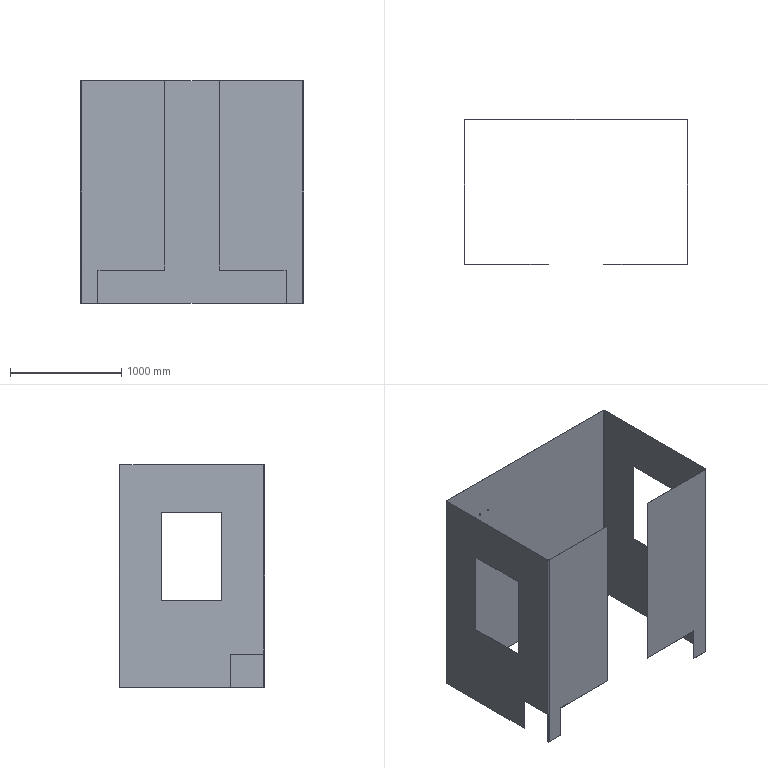Part | SolidWorks | features BaseBody 1 | 1 solid | 61 faces | box 2003 x 1303 x 2000 mm | volume 16327020 mm3 | plane 45 | cylinder 16 | commonest cylinder face diameters 16.5 x8 7 x2 10 x2 17 x2 20 x2